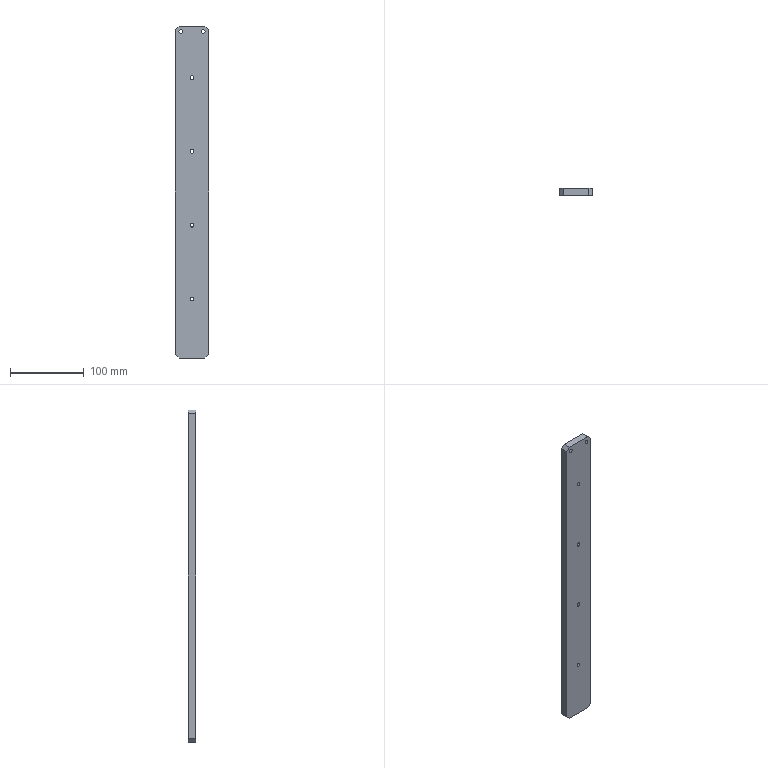Part | NX | 1 solid | 28 faces | box 45 x 10 x 450 mm | volume 198745 mm3 | plane 16 | cylinder 12 | commonest cylinder face diameters 5.3 x6 10 x6
STEP:
#1=CARTESIAN_POINT('',(22.5,10.,220.));
#2=VERTEX_POINT('',#1);
#3=CARTESIAN_POINT('',(22.5,10.,-220.));
#4=VERTEX_POINT('',#3);
#5=CARTESIAN_POINT('',(22.5,10.,225.));
#6=DIRECTION('',(0.,0.,-1.));
#7=VECTOR('',#6,1000.);
#8=LINE('',#5,#7);
#9=EDGE_CURVE('',#2,#4,#8,.T.);
#10=ORIENTED_EDGE('',*,*,#9,.F.);
#11=CARTESIAN_POINT('',(22.5,0.,220.));
#12=VERTEX_POINT('',#11);
#13=CARTESIAN_POINT('',(22.5,10.,220.));
#14=DIRECTION('',(0.,-1.,0.));
#15=VECTOR('',#14,1000.);
#16=LINE('',#13,#15);
#17=EDGE_CURVE('',#2,#12,#16,.T.);
#18=ORIENTED_EDGE('',*,*,#17,.T.);
#19=CARTESIAN_POINT('',(22.5,0.,-220.));
#20=VERTEX_POINT('',#19);
#21=CARTESIAN_POINT('',(22.5,0.,225.));
#22=DIRECTION('',(0.,0.,-1.));
#23=VECTOR('',#22,1000.);
#24=LINE('',#21,#23);
#25=EDGE_CURVE('',#12,#20,#24,.T.);
#26=ORIENTED_EDGE('',*,*,#25,.T.);
#27=CARTESIAN_POINT('',(22.5,10.,-220.));
#28=DIRECTION('',(0.,1.,0.));
#29=VECTOR('',#28,1000.);
#30=LINE('',#27,#29);
#31=EDGE_CURVE('',#20,#4,#30,.T.);
#32=ORIENTED_EDGE('',*,*,#31,.T.);
#33=EDGE_LOOP('',(#10,#18,#26,#32));
#34=FACE_BOUND('',#33,.T.);
#35=CARTESIAN_POINT('',(22.5,10.,225.));
#36=DIRECTION('',(-1.,0.,0.));
#37=DIRECTION('',(0.,0.,1.));
#38=AXIS2_PLACEMENT_3D('',#35,#36,#37);
#39=PLANE('',#38);
#40=ADVANCED_FACE('',(#34),#39,.F.);
#41=CARTESIAN_POINT('',(17.5,10.,-225.));
#42=VERTEX_POINT('',#41);
#43=CARTESIAN_POINT('',(-17.5,10.,-225.));
#44=VERTEX_POINT('',#43);
#45=CARTESIAN_POINT('',(-22.5,10.,-225.));
#46=DIRECTION('',(-1.,0.,0.));
#47=VECTOR('',#46,1000.);
#48=LINE('',#45,#47);
#49=EDGE_CURVE('',#42,#44,#48,.T.);
#50=ORIENTED_EDGE('',*,*,#49,.F.);
#51=CARTESIAN_POINT('',(17.5,0.,-225.));
#52=VERTEX_POINT('',#51);
#53=CARTESIAN_POINT('',(17.5,10.,-225.));
#54=DIRECTION('',(0.,-1.,0.));
#55=VECTOR('',#54,1000.);
#56=LINE('',#53,#55);
#57=EDGE_CURVE('',#42,#52,#56,.T.);
#58=ORIENTED_EDGE('',*,*,#57,.T.);
#59=CARTESIAN_POINT('',(-17.5,0.,-225.));
#60=VERTEX_POINT('',#59);
#61=CARTESIAN_POINT('',(-22.5,0.,-225.));
#62=DIRECTION('',(-1.,0.,0.));
#63=VECTOR('',#62,1000.);
#64=LINE('',#61,#63);
#65=EDGE_CURVE('',#52,#60,#64,.T.);
#66=ORIENTED_EDGE('',*,*,#65,.T.);
#67=CARTESIAN_POINT('',(-17.5,10.,-225.));
#68=DIRECTION('',(0.,1.,0.));
#69=VECTOR('',#68,1000.);
#70=LINE('',#67,#69);
#71=EDGE_CURVE('',#60,#44,#70,.T.);
#72=ORIENTED_EDGE('',*,*,#71,.T.);
#73=EDGE_LOOP('',(#50,#58,#66,#72));
#74=FACE_BOUND('',#73,.T.);
#75=CARTESIAN_POINT('',(-22.5,10.,-225.));
#76=DIRECTION('',(0.,0.,1.));
#77=DIRECTION('',(1.,0.,0.));
#78=AXIS2_PLACEMENT_3D('',#75,#76,#77);
#79=PLANE('',#78);
#80=ADVANCED_FACE('',(#74),#79,.F.);
#81=CARTESIAN_POINT('',(-22.5,0.,-220.));
#82=VERTEX_POINT('',#81);
#83=CARTESIAN_POINT('',(-22.5,0.,220.));
#84=VERTEX_POINT('',#83);
#85=CARTESIAN_POINT('',(-22.5,0.,225.));
#86=DIRECTION('',(0.,0.,1.));
#87=VECTOR('',#86,1000.);
#88=LINE('',#85,#87);
#89=EDGE_CURVE('',#82,#84,#88,.T.);
#90=ORIENTED_EDGE('',*,*,#89,.T.);
#91=CARTESIAN_POINT('',(-22.5,10.,220.));
#92=VERTEX_POINT('',#91);
#93=CARTESIAN_POINT('',(-22.5,10.,220.));
#94=DIRECTION('',(0.,1.,0.));
#95=VECTOR('',#94,1000.);
#96=LINE('',#93,#95);
#97=EDGE_CURVE('',#84,#92,#96,.T.);
#98=ORIENTED_EDGE('',*,*,#97,.T.);
#99=CARTESIAN_POINT('',(-22.5,10.,-220.));
#100=VERTEX_POINT('',#99);
#101=CARTESIAN_POINT('',(-22.5,10.,225.));
#102=DIRECTION('',(0.,0.,1.));
#103=VECTOR('',#102,1000.);
#104=LINE('',#101,#103);
#105=EDGE_CURVE('',#100,#92,#104,.T.);
#106=ORIENTED_EDGE('',*,*,#105,.F.);
#107=CARTESIAN_POINT('',(-22.5,10.,-220.));
#108=DIRECTION('',(0.,-1.,0.));
#109=VECTOR('',#108,1000.);
#110=LINE('',#107,#109);
#111=EDGE_CURVE('',#100,#82,#110,.T.);
#112=ORIENTED_EDGE('',*,*,#111,.T.);
#113=EDGE_LOOP('',(#90,#98,#106,#112));
#114=FACE_BOUND('',#113,.T.);
#115=CARTESIAN_POINT('',(-22.5,10.,225.));
#116=DIRECTION('',(1.,0.,0.));
#117=DIRECTION('',(0.,0.,-1.));
#118=AXIS2_PLACEMENT_3D('',#115,#116,#117);
#119=PLANE('',#118);
#120=ADVANCED_FACE('',(#114),#119,.F.);
#121=CARTESIAN_POINT('',(-17.5,10.,225.));
#122=VERTEX_POINT('',#121);
#123=CARTESIAN_POINT('',(17.5,10.,225.));
#124=VERTEX_POINT('',#123);
#125=CARTESIAN_POINT('',(-22.5,10.,225.));
#126=DIRECTION('',(1.,0.,0.));
#127=VECTOR('',#126,1000.);
#128=LINE('',#125,#127);
#129=EDGE_CURVE('',#122,#124,#128,.T.);
#130=ORIENTED_EDGE('',*,*,#129,.F.);
#131=CARTESIAN_POINT('',(-17.5,0.,225.));
#132=VERTEX_POINT('',#131);
#133=CARTESIAN_POINT('',(-17.5,10.,225.));
#134=DIRECTION('',(0.,-1.,0.));
#135=VECTOR('',#134,1000.);
#136=LINE('',#133,#135);
#137=EDGE_CURVE('',#122,#132,#136,.T.);
#138=ORIENTED_EDGE('',*,*,#137,.T.);
#139=CARTESIAN_POINT('',(17.5,0.,225.));
#140=VERTEX_POINT('',#139);
#141=CARTESIAN_POINT('',(-22.5,0.,225.));
#142=DIRECTION('',(1.,0.,0.));
#143=VECTOR('',#142,1000.);
#144=LINE('',#141,#143);
#145=EDGE_CURVE('',#132,#140,#144,.T.);
#146=ORIENTED_EDGE('',*,*,#145,.T.);
#147=CARTESIAN_POINT('',(17.5,10.,225.));
#148=DIRECTION('',(0.,1.,0.));
#149=VECTOR('',#148,1000.);
#150=LINE('',#147,#149);
#151=EDGE_CURVE('',#140,#124,#150,.T.);
#152=ORIENTED_EDGE('',*,*,#151,.T.);
#153=EDGE_LOOP('',(#130,#138,#146,#152));
#154=FACE_BOUND('',#153,.T.);
#155=CARTESIAN_POINT('',(-22.5,10.,225.));
#156=DIRECTION('',(0.,0.,-1.));
#157=DIRECTION('',(-1.,0.,0.));
#158=AXIS2_PLACEMENT_3D('',#155,#156,#157);
#159=PLANE('',#158);
#160=ADVANCED_FACE('',(#154),#159,.F.);
#161=CARTESIAN_POINT('',(0.,10.,-140.));
#162=VERTEX_POINT('',#161);
#163=CARTESIAN_POINT('',(0.,10.,-145.));
#164=DIRECTION('',(0.,1.,0.));
#165=DIRECTION('',(0.,0.,1.));
#166=AXIS2_PLACEMENT_3D('',#163,#164,#165);
#167=CIRCLE('',#166,5.);
#168=EDGE_CURVE('',#162,#162,#167,.T.);
#169=ORIENTED_EDGE('',*,*,#168,.F.);
#170=EDGE_LOOP('',(#169));
#171=FACE_BOUND('',#170,.T.);
#172=CARTESIAN_POINT('',(0.,10.,-40.));
#173=VERTEX_POINT('',#172);
#174=CARTESIAN_POINT('',(0.,10.,-45.));
#175=DIRECTION('',(0.,1.,0.));
#176=DIRECTION('',(0.,0.,1.));
#177=AXIS2_PLACEMENT_3D('',#174,#175,#176);
#178=CIRCLE('',#177,5.);
#179=EDGE_CURVE('',#173,#173,#178,.T.);
#180=ORIENTED_EDGE('',*,*,#179,.F.);
#181=EDGE_LOOP('',(#180));
#182=FACE_BOUND('',#181,.T.);
#183=CARTESIAN_POINT('',(0.,10.,60.));
#184=VERTEX_POINT('',#183);
#185=CARTESIAN_POINT('',(0.,10.,55.));
#186=DIRECTION('',(0.,1.,0.));
#187=DIRECTION('',(0.,0.,1.));
#188=AXIS2_PLACEMENT_3D('',#185,#186,#187);
#189=CIRCLE('',#188,5.);
#190=EDGE_CURVE('',#184,#184,#189,.T.);
#191=ORIENTED_EDGE('',*,*,#190,.F.);
#192=EDGE_LOOP('',(#191));
#193=FACE_BOUND('',#192,.T.);
#194=CARTESIAN_POINT('',(0.,10.,160.));
#195=VERTEX_POINT('',#194);
#196=CARTESIAN_POINT('',(0.,10.,155.));
#197=DIRECTION('',(0.,1.,0.));
#198=DIRECTION('',(0.,0.,1.));
#199=AXIS2_PLACEMENT_3D('',#196,#197,#198);
#200=CIRCLE('',#199,5.);
#201=EDGE_CURVE('',#195,#195,#200,.T.);
#202=ORIENTED_EDGE('',*,*,#201,.F.);
#203=EDGE_LOOP('',(#202));
#204=FACE_BOUND('',#203,.T.);
#205=CARTESIAN_POINT('',(-15.,10.,222.5));
#206=VERTEX_POINT('',#205);
#207=CARTESIAN_POINT('',(-15.,10.,217.5));
#208=DIRECTION('',(0.,1.,0.));
#209=DIRECTION('',(0.,0.,1.));
#210=AXIS2_PLACEMENT_3D('',#207,#208,#209);
#211=CIRCLE('',#210,5.);
#212=EDGE_CURVE('',#206,#206,#211,.T.);
#213=ORIENTED_EDGE('',*,*,#212,.F.);
#214=EDGE_LOOP('',(#213));
#215=FACE_BOUND('',#214,.T.);
#216=CARTESIAN_POINT('',(15.,10.,222.5));
#217=VERTEX_POINT('',#216);
#218=CARTESIAN_POINT('',(15.,10.,217.5));
#219=DIRECTION('',(0.,1.,0.));
#220=DIRECTION('',(0.,0.,1.));
#221=AXIS2_PLACEMENT_3D('',#218,#219,#220);
#222=CIRCLE('',#221,5.);
#223=EDGE_CURVE('',#217,#217,#222,.T.);
#224=ORIENTED_EDGE('',*,*,#223,.F.);
#225=EDGE_LOOP('',(#224));
#226=FACE_BOUND('',#225,.T.);
#227=ORIENTED_EDGE('',*,*,#105,.T.);
#228=CARTESIAN_POINT('',(-17.5,10.,225.));
#229=DIRECTION('',(-0.7071,0.,-0.7071));
#230=VECTOR('',#229,1000.);
#231=LINE('',#228,#230);
#232=EDGE_CURVE('',#92,#122,#231,.F.);
#233=ORIENTED_EDGE('',*,*,#232,.T.);
#234=ORIENTED_EDGE('',*,*,#129,.T.);
#235=CARTESIAN_POINT('',(22.5,10.,220.));
#236=DIRECTION('',(-0.7071,0.,0.7071));
#237=VECTOR('',#236,1000.);
#238=LINE('',#235,#237);
#239=EDGE_CURVE('',#124,#2,#238,.F.);
#240=ORIENTED_EDGE('',*,*,#239,.T.);
#241=ORIENTED_EDGE('',*,*,#9,.T.);
#242=CARTESIAN_POINT('',(17.5,10.,-225.));
#243=DIRECTION('',(0.7071,0.,0.7071));
#244=VECTOR('',#243,1000.);
#245=LINE('',#242,#244);
#246=EDGE_CURVE('',#4,#42,#245,.F.);
#247=ORIENTED_EDGE('',*,*,#246,.T.);
#248=ORIENTED_EDGE('',*,*,#49,.T.);
#249=CARTESIAN_POINT('',(-22.5,10.,-220.));
#250=DIRECTION('',(0.7071,0.,-0.7071));
#251=VECTOR('',#250,1000.);
#252=LINE('',#249,#251);
#253=EDGE_CURVE('',#44,#100,#252,.F.);
#254=ORIENTED_EDGE('',*,*,#253,.T.);
#255=EDGE_LOOP('',(#227,#233,#234,#240,#241,#247,#248,#254));
#256=FACE_BOUND('',#255,.T.);
#257=CARTESIAN_POINT('',(0.,10.,0.));
#258=DIRECTION('',(0.,-1.,0.));
#259=DIRECTION('',(0.,0.,-1.));
#260=AXIS2_PLACEMENT_3D('',#257,#258,#259);
#261=PLANE('',#260);
#262=ADVANCED_FACE('',(#171,#182,#193,#204,#215,#226,#256),#261,.F.);
#263=CARTESIAN_POINT('',(0.,0.,-142.35));
#264=VERTEX_POINT('',#263);
#265=CARTESIAN_POINT('',(0.,0.,-145.));
#266=DIRECTION('',(0.,1.,0.));
#267=DIRECTION('',(0.,0.,1.));
#268=AXIS2_PLACEMENT_3D('',#265,#266,#267);
#269=CIRCLE('',#268,2.65);
#270=EDGE_CURVE('',#264,#264,#269,.T.);
#271=ORIENTED_EDGE('',*,*,#270,.T.);
#272=EDGE_LOOP('',(#271));
#273=FACE_BOUND('',#272,.T.);
#274=CARTESIAN_POINT('',(0.,0.,-42.35));
#275=VERTEX_POINT('',#274);
#276=CARTESIAN_POINT('',(0.,0.,-45.));
#277=DIRECTION('',(0.,1.,0.));
#278=DIRECTION('',(0.,0.,1.));
#279=AXIS2_PLACEMENT_3D('',#276,#277,#278);
#280=CIRCLE('',#279,2.65);
#281=EDGE_CURVE('',#275,#275,#280,.T.);
#282=ORIENTED_EDGE('',*,*,#281,.T.);
#283=EDGE_LOOP('',(#282));
#284=FACE_BOUND('',#283,.T.);
#285=CARTESIAN_POINT('',(0.,0.,57.65));
#286=VERTEX_POINT('',#285);
#287=CARTESIAN_POINT('',(0.,0.,55.));
#288=DIRECTION('',(0.,1.,0.));
#289=DIRECTION('',(0.,0.,1.));
#290=AXIS2_PLACEMENT_3D('',#287,#288,#289);
#291=CIRCLE('',#290,2.65);
#292=EDGE_CURVE('',#286,#286,#291,.T.);
#293=ORIENTED_EDGE('',*,*,#292,.T.);
#294=EDGE_LOOP('',(#293));
#295=FACE_BOUND('',#294,.T.);
#296=CARTESIAN_POINT('',(0.,0.,157.65));
#297=VERTEX_POINT('',#296);
#298=CARTESIAN_POINT('',(0.,0.,155.));
#299=DIRECTION('',(0.,1.,0.));
#300=DIRECTION('',(0.,0.,1.));
#301=AXIS2_PLACEMENT_3D('',#298,#299,#300);
#302=CIRCLE('',#301,2.65);
#303=EDGE_CURVE('',#297,#297,#302,.T.);
#304=ORIENTED_EDGE('',*,*,#303,.T.);
#305=EDGE_LOOP('',(#304));
#306=FACE_BOUND('',#305,.T.);
#307=CARTESIAN_POINT('',(-15.,0.,220.15));
#308=VERTEX_POINT('',#307);
#309=CARTESIAN_POINT('',(-15.,0.,217.5));
#310=DIRECTION('',(0.,1.,0.));
#311=DIRECTION('',(0.,0.,1.));
#312=AXIS2_PLACEMENT_3D('',#309,#310,#311);
#313=CIRCLE('',#312,2.65);
#314=EDGE_CURVE('',#308,#308,#313,.T.);
#315=ORIENTED_EDGE('',*,*,#314,.T.);
#316=EDGE_LOOP('',(#315));
#317=FACE_BOUND('',#316,.T.);
#318=CARTESIAN_POINT('',(15.,0.,220.15));
#319=VERTEX_POINT('',#318);
#320=CARTESIAN_POINT('',(15.,0.,217.5));
#321=DIRECTION('',(0.,1.,0.));
#322=DIRECTION('',(0.,0.,1.));
#323=AXIS2_PLACEMENT_3D('',#320,#321,#322);
#324=CIRCLE('',#323,2.65);
#325=EDGE_CURVE('',#319,#319,#324,.T.);
#326=ORIENTED_EDGE('',*,*,#325,.T.);
#327=EDGE_LOOP('',(#326));
#328=FACE_BOUND('',#327,.T.);
#329=ORIENTED_EDGE('',*,*,#145,.F.);
#330=CARTESIAN_POINT('',(-121.25,0.,121.25));
#331=DIRECTION('',(0.7071,0.,0.7071));
#332=VECTOR('',#331,1000.);
#333=LINE('',#330,#332);
#334=EDGE_CURVE('',#132,#84,#333,.F.);
#335=ORIENTED_EDGE('',*,*,#334,.T.);
#336=ORIENTED_EDGE('',*,*,#89,.F.);
#337=CARTESIAN_POINT('',(-121.25,0.,-121.25));
#338=DIRECTION('',(-0.7071,0.,0.7071));
#339=VECTOR('',#338,1000.);
#340=LINE('',#337,#339);
#341=EDGE_CURVE('',#82,#60,#340,.F.);
#342=ORIENTED_EDGE('',*,*,#341,.T.);
#343=ORIENTED_EDGE('',*,*,#65,.F.);
#344=CARTESIAN_POINT('',(121.25,0.,-121.25));
#345=DIRECTION('',(-0.7071,0.,-0.7071));
#346=VECTOR('',#345,1000.);
#347=LINE('',#344,#346);
#348=EDGE_CURVE('',#52,#20,#347,.F.);
#349=ORIENTED_EDGE('',*,*,#348,.T.);
#350=ORIENTED_EDGE('',*,*,#25,.F.);
#351=CARTESIAN_POINT('',(121.25,0.,121.25));
#352=DIRECTION('',(0.7071,0.,-0.7071));
#353=VECTOR('',#352,1000.);
#354=LINE('',#351,#353);
#355=EDGE_CURVE('',#12,#140,#354,.F.);
#356=ORIENTED_EDGE('',*,*,#355,.T.);
#357=EDGE_LOOP('',(#329,#335,#336,#342,#343,#349,#350,#356));
#358=FACE_BOUND('',#357,.T.);
#359=CARTESIAN_POINT('',(0.,0.,0.));
#360=DIRECTION('',(0.,-1.,0.));
#361=DIRECTION('',(0.,0.,-1.));
#362=AXIS2_PLACEMENT_3D('',#359,#360,#361);
#363=PLANE('',#362);
#364=ADVANCED_FACE('',(#273,#284,#295,#306,#317,#328,#358),#363,.T.);
#365=ORIENTED_EDGE('',*,*,#325,.F.);
#366=EDGE_LOOP('',(#365));
#367=FACE_BOUND('',#366,.T.);
#368=CARTESIAN_POINT('',(15.,4.3,220.15));
#369=VERTEX_POINT('',#368);
#370=CARTESIAN_POINT('',(15.,4.3,217.5));
#371=DIRECTION('',(0.,1.,0.));
#372=DIRECTION('',(0.,0.,1.));
#373=AXIS2_PLACEMENT_3D('',#370,#371,#372);
#374=CIRCLE('',#373,2.65);
#375=EDGE_CURVE('',#369,#369,#374,.T.);
#376=ORIENTED_EDGE('',*,*,#375,.T.);
#377=EDGE_LOOP('',(#376));
#378=FACE_BOUND('',#377,.T.);
#379=CARTESIAN_POINT('',(15.,10.,217.5));
#380=DIRECTION('',(0.,1.,0.));
#381=DIRECTION('',(0.,0.,1.));
#382=AXIS2_PLACEMENT_3D('',#379,#380,#381);
#383=CYLINDRICAL_SURFACE('',#382,2.65);
#384=ADVANCED_FACE('',(#367,#378),#383,.F.);
#385=ORIENTED_EDGE('',*,*,#375,.F.);
#386=EDGE_LOOP('',(#385));
#387=FACE_BOUND('',#386,.T.);
#388=CARTESIAN_POINT('',(15.,4.3,222.5));
#389=VERTEX_POINT('',#388);
#390=CARTESIAN_POINT('',(15.,4.3,217.5));
#391=DIRECTION('',(0.,1.,0.));
#392=DIRECTION('',(0.,0.,1.));
#393=AXIS2_PLACEMENT_3D('',#390,#391,#392);
#394=CIRCLE('',#393,5.);
#395=EDGE_CURVE('',#389,#389,#394,.T.);
#396=ORIENTED_EDGE('',*,*,#395,.T.);
#397=EDGE_LOOP('',(#396));
#398=FACE_BOUND('',#397,.T.);
#399=CARTESIAN_POINT('',(17.65,4.3,217.5));
#400=DIRECTION('',(0.,-1.,0.));
#401=DIRECTION('',(0.,0.,-1.));
#402=AXIS2_PLACEMENT_3D('',#399,#400,#401);
#403=PLANE('',#402);
#404=ADVANCED_FACE('',(#387,#398),#403,.F.);
#405=ORIENTED_EDGE('',*,*,#395,.F.);
#406=EDGE_LOOP('',(#405));
#407=FACE_BOUND('',#406,.T.);
#408=ORIENTED_EDGE('',*,*,#223,.T.);
#409=EDGE_LOOP('',(#408));
#410=FACE_BOUND('',#409,.T.);
#411=CARTESIAN_POINT('',(15.,10.,217.5));
#412=DIRECTION('',(0.,1.,0.));
#413=DIRECTION('',(0.,0.,1.));
#414=AXIS2_PLACEMENT_3D('',#411,#412,#413);
#415=CYLINDRICAL_SURFACE('',#414,5.);
#416=ADVANCED_FACE('',(#407,#410),#415,.F.);
#417=ORIENTED_EDGE('',*,*,#314,.F.);
#418=EDGE_LOOP('',(#417));
#419=FACE_BOUND('',#418,.T.);
#420=CARTESIAN_POINT('',(-15.,4.3,220.15));
#421=VERTEX_POINT('',#420);
#422=CARTESIAN_POINT('',(-15.,4.3,217.5));
#423=DIRECTION('',(0.,1.,0.));
#424=DIRECTION('',(0.,0.,1.));
#425=AXIS2_PLACEMENT_3D('',#422,#423,#424);
#426=CIRCLE('',#425,2.65);
#427=EDGE_CURVE('',#421,#421,#426,.T.);
#428=ORIENTED_EDGE('',*,*,#427,.T.);
#429=EDGE_LOOP('',(#428));
#430=FACE_BOUND('',#429,.T.);
#431=CARTESIAN_POINT('',(-15.,10.,217.5));
#432=DIRECTION('',(0.,1.,0.));
#433=DIRECTION('',(0.,0.,1.));
#434=AXIS2_PLACEMENT_3D('',#431,#432,#433);
#435=CYLINDRICAL_SURFACE('',#434,2.65);
#436=ADVANCED_FACE('',(#419,#430),#435,.F.);
#437=ORIENTED_EDGE('',*,*,#427,.F.);
#438=EDGE_LOOP('',(#437));
#439=FACE_BOUND('',#438,.T.);
#440=CARTESIAN_POINT('',(-15.,4.3,222.5));
#441=VERTEX_POINT('',#440);
#442=CARTESIAN_POINT('',(-15.,4.3,217.5));
#443=DIRECTION('',(0.,1.,0.));
#444=DIRECTION('',(0.,0.,1.));
#445=AXIS2_PLACEMENT_3D('',#442,#443,#444);
#446=CIRCLE('',#445,5.);
#447=EDGE_CURVE('',#441,#441,#446,.T.);
#448=ORIENTED_EDGE('',*,*,#447,.T.);
#449=EDGE_LOOP('',(#448));
#450=FACE_BOUND('',#449,.T.);
#451=CARTESIAN_POINT('',(-12.35,4.3,217.5));
#452=DIRECTION('',(0.,-1.,0.));
#453=DIRECTION('',(0.,0.,-1.));
#454=AXIS2_PLACEMENT_3D('',#451,#452,#453);
#455=PLANE('',#454);
#456=ADVANCED_FACE('',(#439,#450),#455,.F.);
#457=ORIENTED_EDGE('',*,*,#447,.F.);
#458=EDGE_LOOP('',(#457));
#459=FACE_BOUND('',#458,.T.);
#460=ORIENTED_EDGE('',*,*,#212,.T.);
#461=EDGE_LOOP('',(#460));
#462=FACE_BOUND('',#461,.T.);
#463=CARTESIAN_POINT('',(-15.,10.,217.5));
#464=DIRECTION('',(0.,1.,0.));
#465=DIRECTION('',(0.,0.,1.));
#466=AXIS2_PLACEMENT_3D('',#463,#464,#465);
#467=CYLINDRICAL_SURFACE('',#466,5.);
#468=ADVANCED_FACE('',(#459,#462),#467,.F.);
#469=ORIENTED_EDGE('',*,*,#303,.F.);
#470=EDGE_LOOP('',(#469));
#471=FACE_BOUND('',#470,.T.);
#472=CARTESIAN_POINT('',(0.,4.3,157.65));
#473=VERTEX_POINT('',#472);
#474=CARTESIAN_POINT('',(0.,4.3,155.));
#475=DIRECTION('',(0.,1.,0.));
#476=DIRECTION('',(0.,0.,1.));
#477=AXIS2_PLACEMENT_3D('',#474,#475,#476);
#478=CIRCLE('',#477,2.65);
#479=EDGE_CURVE('',#473,#473,#478,.T.);
#480=ORIENTED_EDGE('',*,*,#479,.T.);
#481=EDGE_LOOP('',(#480));
#482=FACE_BOUND('',#481,.T.);
#483=CARTESIAN_POINT('',(0.,10.,155.));
#484=DIRECTION('',(0.,1.,0.));
#485=DIRECTION('',(0.,0.,1.));
#486=AXIS2_PLACEMENT_3D('',#483,#484,#485);
#487=CYLINDRICAL_SURFACE('',#486,2.65);
#488=ADVANCED_FACE('',(#471,#482),#487,.F.);
#489=ORIENTED_EDGE('',*,*,#479,.F.);
#490=EDGE_LOOP('',(#489));
#491=FACE_BOUND('',#490,.T.);
#492=CARTESIAN_POINT('',(0.,4.3,160.));
#493=VERTEX_POINT('',#492);
#494=CARTESIAN_POINT('',(0.,4.3,155.));
#495=DIRECTION('',(0.,1.,0.));
#496=DIRECTION('',(0.,0.,1.));
#497=AXIS2_PLACEMENT_3D('',#494,#495,#496);
#498=CIRCLE('',#497,5.);
#499=EDGE_CURVE('',#493,#493,#498,.T.);
#500=ORIENTED_EDGE('',*,*,#499,.T.);
#501=EDGE_LOOP('',(#500));
#502=FACE_BOUND('',#501,.T.);
#503=CARTESIAN_POINT('',(2.65,4.3,155.));
#504=DIRECTION('',(0.,-1.,0.));
#505=DIRECTION('',(0.,0.,-1.));
#506=AXIS2_PLACEMENT_3D('',#503,#504,#505);
#507=PLANE('',#506);
#508=ADVANCED_FACE('',(#491,#502),#507,.F.);
#509=ORIENTED_EDGE('',*,*,#499,.F.);
#510=EDGE_LOOP('',(#509));
#511=FACE_BOUND('',#510,.T.);
#512=ORIENTED_EDGE('',*,*,#201,.T.);
#513=EDGE_LOOP('',(#512));
#514=FACE_BOUND('',#513,.T.);
#515=CARTESIAN_POINT('',(0.,10.,155.));
#516=DIRECTION('',(0.,1.,0.));
#517=DIRECTION('',(0.,0.,1.));
#518=AXIS2_PLACEMENT_3D('',#515,#516,#517);
#519=CYLINDRICAL_SURFACE('',#518,5.);
#520=ADVANCED_FACE('',(#511,#514),#519,.F.);
#521=ORIENTED_EDGE('',*,*,#292,.F.);
#522=EDGE_LOOP('',(#521));
#523=FACE_BOUND('',#522,.T.);
#524=CARTESIAN_POINT('',(0.,4.3,57.65));
#525=VERTEX_POINT('',#524);
#526=CARTESIAN_POINT('',(0.,4.3,55.));
#527=DIRECTION('',(0.,1.,0.));
#528=DIRECTION('',(0.,0.,1.));
#529=AXIS2_PLACEMENT_3D('',#526,#527,#528);
#530=CIRCLE('',#529,2.65);
#531=EDGE_CURVE('',#525,#525,#530,.T.);
#532=ORIENTED_EDGE('',*,*,#531,.T.);
#533=EDGE_LOOP('',(#532));
#534=FACE_BOUND('',#533,.T.);
#535=CARTESIAN_POINT('',(0.,10.,55.));
#536=DIRECTION('',(0.,1.,0.));
#537=DIRECTION('',(0.,0.,1.));
#538=AXIS2_PLACEMENT_3D('',#535,#536,#537);
#539=CYLINDRICAL_SURFACE('',#538,2.65);
#540=ADVANCED_FACE('',(#523,#534),#539,.F.);
#541=ORIENTED_EDGE('',*,*,#531,.F.);
#542=EDGE_LOOP('',(#541));
#543=FACE_BOUND('',#542,.T.);
#544=CARTESIAN_POINT('',(0.,4.3,60.));
#545=VERTEX_POINT('',#544);
#546=CARTESIAN_POINT('',(0.,4.3,55.));
#547=DIRECTION('',(0.,1.,0.));
#548=DIRECTION('',(0.,0.,1.));
#549=AXIS2_PLACEMENT_3D('',#546,#547,#548);
#550=CIRCLE('',#549,5.);
#551=EDGE_CURVE('',#545,#545,#550,.T.);
#552=ORIENTED_EDGE('',*,*,#551,.T.);
#553=EDGE_LOOP('',(#552));
#554=FACE_BOUND('',#553,.T.);
#555=CARTESIAN_POINT('',(2.65,4.3,55.));
#556=DIRECTION('',(0.,-1.,0.));
#557=DIRECTION('',(0.,0.,-1.));
#558=AXIS2_PLACEMENT_3D('',#555,#556,#557);
#559=PLANE('',#558);
#560=ADVANCED_FACE('',(#543,#554),#559,.F.);
#561=ORIENTED_EDGE('',*,*,#551,.F.);
#562=EDGE_LOOP('',(#561));
#563=FACE_BOUND('',#562,.T.);
#564=ORIENTED_EDGE('',*,*,#190,.T.);
#565=EDGE_LOOP('',(#564));
#566=FACE_BOUND('',#565,.T.);
#567=CARTESIAN_POINT('',(0.,10.,55.));
#568=DIRECTION('',(0.,1.,0.));
#569=DIRECTION('',(0.,0.,1.));
#570=AXIS2_PLACEMENT_3D('',#567,#568,#569);
#571=CYLINDRICAL_SURFACE('',#570,5.);
#572=ADVANCED_FACE('',(#563,#566),#571,.F.);
#573=ORIENTED_EDGE('',*,*,#281,.F.);
#574=EDGE_LOOP('',(#573));
#575=FACE_BOUND('',#574,.T.);
#576=CARTESIAN_POINT('',(0.,4.3,-42.35));
#577=VERTEX_POINT('',#576);
#578=CARTESIAN_POINT('',(0.,4.3,-45.));
#579=DIRECTION('',(0.,1.,0.));
#580=DIRECTION('',(0.,0.,1.));
#581=AXIS2_PLACEMENT_3D('',#578,#579,#580);
#582=CIRCLE('',#581,2.65);
#583=EDGE_CURVE('',#577,#577,#582,.T.);
#584=ORIENTED_EDGE('',*,*,#583,.T.);
#585=EDGE_LOOP('',(#584));
#586=FACE_BOUND('',#585,.T.);
#587=CARTESIAN_POINT('',(0.,10.,-45.));
#588=DIRECTION('',(0.,1.,0.));
#589=DIRECTION('',(0.,0.,1.));
#590=AXIS2_PLACEMENT_3D('',#587,#588,#589);
#591=CYLINDRICAL_SURFACE('',#590,2.65);
#592=ADVANCED_FACE('',(#575,#586),#591,.F.);
#593=ORIENTED_EDGE('',*,*,#583,.F.);
#594=EDGE_LOOP('',(#593));
#595=FACE_BOUND('',#594,.T.);
#596=CARTESIAN_POINT('',(0.,4.3,-40.));
#597=VERTEX_POINT('',#596);
#598=CARTESIAN_POINT('',(0.,4.3,-45.));
#599=DIRECTION('',(0.,1.,0.));
#600=DIRECTION('',(0.,0.,1.));
#601=AXIS2_PLACEMENT_3D('',#598,#599,#600);
#602=CIRCLE('',#601,5.);
#603=EDGE_CURVE('',#597,#597,#602,.T.);
#604=ORIENTED_EDGE('',*,*,#603,.T.);
#605=EDGE_LOOP('',(#604));
#606=FACE_BOUND('',#605,.T.);
#607=CARTESIAN_POINT('',(2.65,4.3,-45.));
#608=DIRECTION('',(0.,-1.,0.));
#609=DIRECTION('',(0.,0.,-1.));
#610=AXIS2_PLACEMENT_3D('',#607,#608,#609);
#611=PLANE('',#610);
#612=ADVANCED_FACE('',(#595,#606),#611,.F.);
#613=ORIENTED_EDGE('',*,*,#603,.F.);
#614=EDGE_LOOP('',(#613));
#615=FACE_BOUND('',#614,.T.);
#616=ORIENTED_EDGE('',*,*,#179,.T.);
#617=EDGE_LOOP('',(#616));
#618=FACE_BOUND('',#617,.T.);
#619=CARTESIAN_POINT('',(0.,10.,-45.));
#620=DIRECTION('',(0.,1.,0.));
#621=DIRECTION('',(0.,0.,1.));
#622=AXIS2_PLACEMENT_3D('',#619,#620,#621);
#623=CYLINDRICAL_SURFACE('',#622,5.);
#624=ADVANCED_FACE('',(#615,#618),#623,.F.);
#625=ORIENTED_EDGE('',*,*,#270,.F.);
#626=EDGE_LOOP('',(#625));
#627=FACE_BOUND('',#626,.T.);
#628=CARTESIAN_POINT('',(0.,4.3,-142.35));
#629=VERTEX_POINT('',#628);
#630=CARTESIAN_POINT('',(0.,4.3,-145.));
#631=DIRECTION('',(0.,1.,0.));
#632=DIRECTION('',(0.,0.,1.));
#633=AXIS2_PLACEMENT_3D('',#630,#631,#632);
#634=CIRCLE('',#633,2.65);
#635=EDGE_CURVE('',#629,#629,#634,.T.);
#636=ORIENTED_EDGE('',*,*,#635,.T.);
#637=EDGE_LOOP('',(#636));
#638=FACE_BOUND('',#637,.T.);
#639=CARTESIAN_POINT('',(0.,10.,-145.));
#640=DIRECTION('',(0.,1.,0.));
#641=DIRECTION('',(0.,0.,1.));
#642=AXIS2_PLACEMENT_3D('',#639,#640,#641);
#643=CYLINDRICAL_SURFACE('',#642,2.65);
#644=ADVANCED_FACE('',(#627,#638),#643,.F.);
#645=ORIENTED_EDGE('',*,*,#635,.F.);
#646=EDGE_LOOP('',(#645));
#647=FACE_BOUND('',#646,.T.);
#648=CARTESIAN_POINT('',(0.,4.3,-140.));
#649=VERTEX_POINT('',#648);
#650=CARTESIAN_POINT('',(0.,4.3,-145.));
#651=DIRECTION('',(0.,1.,0.));
#652=DIRECTION('',(0.,0.,1.));
#653=AXIS2_PLACEMENT_3D('',#650,#651,#652);
#654=CIRCLE('',#653,5.);
#655=EDGE_CURVE('',#649,#649,#654,.T.);
#656=ORIENTED_EDGE('',*,*,#655,.T.);
#657=EDGE_LOOP('',(#656));
#658=FACE_BOUND('',#657,.T.);
#659=CARTESIAN_POINT('',(2.65,4.3,-145.));
#660=DIRECTION('',(0.,-1.,0.));
#661=DIRECTION('',(0.,0.,-1.));
#662=AXIS2_PLACEMENT_3D('',#659,#660,#661);
#663=PLANE('',#662);
#664=ADVANCED_FACE('',(#647,#658),#663,.F.);
#665=ORIENTED_EDGE('',*,*,#655,.F.);
#666=EDGE_LOOP('',(#665));
#667=FACE_BOUND('',#666,.T.);
#668=ORIENTED_EDGE('',*,*,#168,.T.);
#669=EDGE_LOOP('',(#668));
#670=FACE_BOUND('',#669,.T.);
#671=CARTESIAN_POINT('',(0.,10.,-145.));
#672=DIRECTION('',(0.,1.,0.));
#673=DIRECTION('',(0.,0.,1.));
#674=AXIS2_PLACEMENT_3D('',#671,#672,#673);
#675=CYLINDRICAL_SURFACE('',#674,5.);
#676=ADVANCED_FACE('',(#667,#670),#675,.F.);
#677=ORIENTED_EDGE('',*,*,#232,.F.);
#678=ORIENTED_EDGE('',*,*,#97,.F.);
#679=ORIENTED_EDGE('',*,*,#334,.F.);
#680=ORIENTED_EDGE('',*,*,#137,.F.);
#681=EDGE_LOOP('',(#677,#678,#679,#680));
#682=FACE_BOUND('',#681,.T.);
#683=CARTESIAN_POINT('',(-17.5,10.,225.));
#684=DIRECTION('',(0.7071,0.,-0.7071));
#685=DIRECTION('',(0.,-1.,0.));
#686=AXIS2_PLACEMENT_3D('',#683,#684,#685);
#687=PLANE('',#686);
#688=ADVANCED_FACE('',(#682),#687,.F.);
#689=ORIENTED_EDGE('',*,*,#239,.F.);
#690=ORIENTED_EDGE('',*,*,#151,.F.);
#691=ORIENTED_EDGE('',*,*,#355,.F.);
#692=ORIENTED_EDGE('',*,*,#17,.F.);
#693=EDGE_LOOP('',(#689,#690,#691,#692));
#694=FACE_BOUND('',#693,.T.);
#695=CARTESIAN_POINT('',(22.5,10.,220.));
#696=DIRECTION('',(-0.7071,0.,-0.7071));
#697=DIRECTION('',(0.,-1.,0.));
#698=AXIS2_PLACEMENT_3D('',#695,#696,#697);
#699=PLANE('',#698);
#700=ADVANCED_FACE('',(#694),#699,.F.);
#701=ORIENTED_EDGE('',*,*,#246,.F.);
#702=ORIENTED_EDGE('',*,*,#31,.F.);
#703=ORIENTED_EDGE('',*,*,#348,.F.);
#704=ORIENTED_EDGE('',*,*,#57,.F.);
#705=EDGE_LOOP('',(#701,#702,#703,#704));
#706=FACE_BOUND('',#705,.T.);
#707=CARTESIAN_POINT('',(17.5,10.,-225.));
#708=DIRECTION('',(-0.7071,0.,0.7071));
#709=DIRECTION('',(0.,-1.,0.));
#710=AXIS2_PLACEMENT_3D('',#707,#708,#709);
#711=PLANE('',#710);
#712=ADVANCED_FACE('',(#706),#711,.F.);
#713=ORIENTED_EDGE('',*,*,#253,.F.);
#714=ORIENTED_EDGE('',*,*,#71,.F.);
#715=ORIENTED_EDGE('',*,*,#341,.F.);
#716=ORIENTED_EDGE('',*,*,#111,.F.);
#717=EDGE_LOOP('',(#713,#714,#715,#716));
#718=FACE_BOUND('',#717,.T.);
#719=CARTESIAN_POINT('',(-22.5,10.,-220.));
#720=DIRECTION('',(0.7071,0.,0.7071));
#721=DIRECTION('',(0.,-1.,0.));
#722=AXIS2_PLACEMENT_3D('',#719,#720,#721);
#723=PLANE('',#722);
#724=ADVANCED_FACE('',(#718),#723,.F.);
#725=CLOSED_SHELL('',(#40,#80,#120,#160,#262,#364,#384,#404,#416,#436,#456,#468,#488,#508,#520,#540,#560,#572,#592,#612,#624,#644,#664,#676,#688,#700,#712,#724));
#726=MANIFOLD_SOLID_BREP('',#725);
#727=(LENGTH_UNIT()NAMED_UNIT(*)SI_UNIT(.MILLI.,.METRE.));
#728=UNCERTAINTY_MEASURE_WITH_UNIT(LENGTH_MEASURE(0.00001),#727,'','');
#729=(NAMED_UNIT(*)PLANE_ANGLE_UNIT()SI_UNIT($,.RADIAN.));
#730=(NAMED_UNIT(*)SI_UNIT($,.STERADIAN.)SOLID_ANGLE_UNIT());
#731=(GEOMETRIC_REPRESENTATION_CONTEXT(3)GLOBAL_UNCERTAINTY_ASSIGNED_CONTEXT((#728))GLOBAL_UNIT_ASSIGNED_CONTEXT((#727,#729,#730))REPRESENTATION_CONTEXT('',''));
#732=ADVANCED_BREP_SHAPE_REPRESENTATION('',(#726),#731);